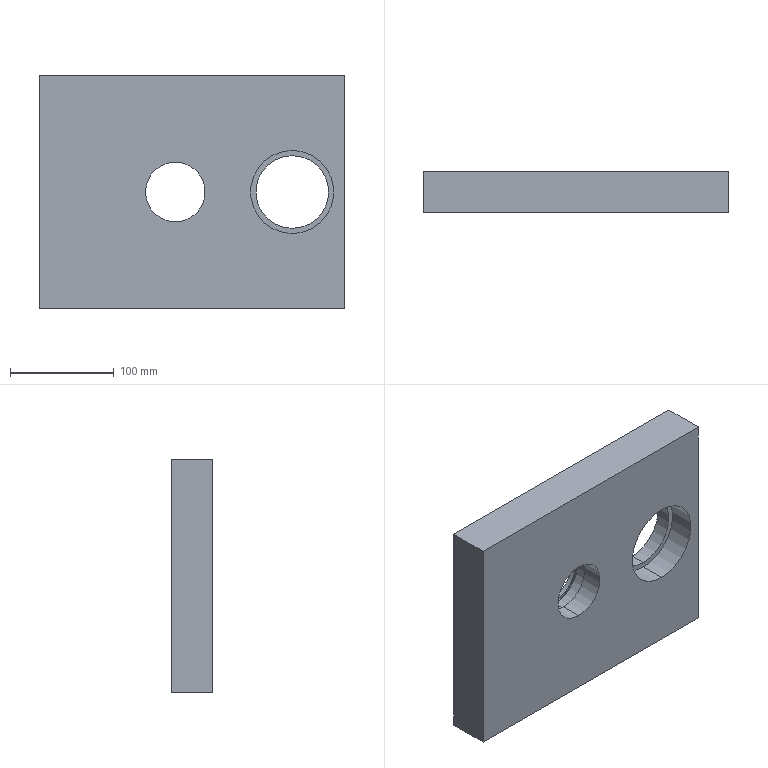Part | SolidWorks | features Cut 3, ICE 2, Extrusion 1 | 1 solid | 22 faces | box 293 x 40 x 225 mm | volume 2341161 mm3 | cylinder 12 | plane 10 | commonest cylinder face diameters 62 x4 57.4 x2 65 x2 70 x2 80 x2
STEP:
#1=CARTESIAN_POINT('',(-16.,32.8,-32.5));
#2=VERTEX_POINT('',#1);
#3=CARTESIAN_POINT('',(-16.,32.8,32.5));
#4=VERTEX_POINT('',#3);
#5=CARTESIAN_POINT('',(-16.,32.8,0.));
#6=DIRECTION('',(0.,1.,0.));
#7=DIRECTION('',(0.,0.,1.));
#8=AXIS2_PLACEMENT_3D('',#5,#6,#7);
#9=CIRCLE('',#8,32.5);
#10=EDGE_CURVE('',#2,#4,#9,.T.);
#11=ORIENTED_EDGE('',*,*,#10,.F.);
#12=CARTESIAN_POINT('',(-16.,35.,-32.5));
#13=VERTEX_POINT('',#12);
#14=CARTESIAN_POINT('',(-16.,32.8,-32.5));
#15=DIRECTION('',(0.,1.,0.));
#16=VECTOR('',#15,1000.);
#17=LINE('',#14,#16);
#18=EDGE_CURVE('',#2,#13,#17,.T.);
#19=ORIENTED_EDGE('',*,*,#18,.T.);
#20=CARTESIAN_POINT('',(-16.,35.,32.5));
#21=VERTEX_POINT('',#20);
#22=CARTESIAN_POINT('',(-16.,35.,0.));
#23=DIRECTION('',(0.,1.,0.));
#24=DIRECTION('',(0.,0.,1.));
#25=AXIS2_PLACEMENT_3D('',#22,#23,#24);
#26=CIRCLE('',#25,32.5);
#27=EDGE_CURVE('',#13,#21,#26,.T.);
#28=ORIENTED_EDGE('',*,*,#27,.T.);
#29=CARTESIAN_POINT('',(-16.,32.8,32.5));
#30=DIRECTION('',(0.,1.,0.));
#31=VECTOR('',#30,1000.);
#32=LINE('',#29,#31);
#33=EDGE_CURVE('',#4,#21,#32,.T.);
#34=ORIENTED_EDGE('',*,*,#33,.F.);
#35=EDGE_LOOP('',(#11,#19,#28,#34));
#36=FACE_OUTER_BOUND('',#35,.T.);
#37=CARTESIAN_POINT('',(-16.,32.8,0.));
#38=DIRECTION('',(0.,1.,0.));
#39=DIRECTION('',(0.,0.,1.));
#40=AXIS2_PLACEMENT_3D('',#37,#38,#39);
#41=CYLINDRICAL_SURFACE('',#40,32.5);
#42=ADVANCED_FACE('',(#36),#41,.F.);
#43=CARTESIAN_POINT('',(-16.,35.,31.));
#44=VERTEX_POINT('',#43);
#45=CARTESIAN_POINT('',(-16.,35.,-31.));
#46=VERTEX_POINT('',#45);
#47=CARTESIAN_POINT('',(-16.,35.,0.));
#48=DIRECTION('',(0.,-1.,0.));
#49=DIRECTION('',(0.,0.,1.));
#50=AXIS2_PLACEMENT_3D('',#47,#48,#49);
#51=CIRCLE('',#50,31.);
#52=EDGE_CURVE('',#44,#46,#51,.T.);
#53=ORIENTED_EDGE('',*,*,#52,.T.);
#54=CARTESIAN_POINT('',(-16.,40.,-31.));
#55=VERTEX_POINT('',#54);
#56=CARTESIAN_POINT('',(-16.,20.8,-31.));
#57=DIRECTION('',(0.,1.,0.));
#58=VECTOR('',#57,1000.);
#59=LINE('',#56,#58);
#60=EDGE_CURVE('',#46,#55,#59,.T.);
#61=ORIENTED_EDGE('',*,*,#60,.T.);
#62=CARTESIAN_POINT('',(-16.,40.,31.));
#63=VERTEX_POINT('',#62);
#64=CARTESIAN_POINT('',(-16.,40.,0.));
#65=DIRECTION('',(0.,1.,0.));
#66=DIRECTION('',(0.,0.,1.));
#67=AXIS2_PLACEMENT_3D('',#64,#65,#66);
#68=CIRCLE('',#67,31.);
#69=EDGE_CURVE('',#55,#63,#68,.T.);
#70=ORIENTED_EDGE('',*,*,#69,.T.);
#71=CARTESIAN_POINT('',(-16.,20.8,31.));
#72=DIRECTION('',(0.,1.,0.));
#73=VECTOR('',#72,1000.);
#74=LINE('',#71,#73);
#75=EDGE_CURVE('',#44,#63,#74,.T.);
#76=ORIENTED_EDGE('',*,*,#75,.F.);
#77=EDGE_LOOP('',(#53,#61,#70,#76));
#78=FACE_OUTER_BOUND('',#77,.T.);
#79=CARTESIAN_POINT('',(-16.,20.8,0.));
#80=DIRECTION('',(0.,1.,0.));
#81=DIRECTION('',(0.,0.,1.));
#82=AXIS2_PLACEMENT_3D('',#79,#80,#81);
#83=CYLINDRICAL_SURFACE('',#82,31.);
#84=ADVANCED_FACE('',(#78),#83,.F.);
#85=CARTESIAN_POINT('',(96.5,40.,35.));
#86=VERTEX_POINT('',#85);
#87=CARTESIAN_POINT('',(96.5,40.,-35.));
#88=VERTEX_POINT('',#87);
#89=CARTESIAN_POINT('',(96.5,40.,0.));
#90=DIRECTION('',(0.,-1.,0.));
#91=DIRECTION('',(0.,0.,-1.));
#92=AXIS2_PLACEMENT_3D('',#89,#90,#91);
#93=CIRCLE('',#92,35.);
#94=EDGE_CURVE('',#86,#88,#93,.T.);
#95=ORIENTED_EDGE('',*,*,#94,.F.);
#96=CARTESIAN_POINT('',(96.5,25.,35.));
#97=VERTEX_POINT('',#96);
#98=CARTESIAN_POINT('',(96.5,40.,35.));
#99=DIRECTION('',(0.,-1.,0.));
#100=VECTOR('',#99,1000.);
#101=LINE('',#98,#100);
#102=EDGE_CURVE('',#86,#97,#101,.T.);
#103=ORIENTED_EDGE('',*,*,#102,.T.);
#104=CARTESIAN_POINT('',(96.5,25.,-35.));
#105=VERTEX_POINT('',#104);
#106=CARTESIAN_POINT('',(96.5,25.,0.));
#107=DIRECTION('',(0.,-1.,0.));
#108=DIRECTION('',(0.,0.,-1.));
#109=AXIS2_PLACEMENT_3D('',#106,#107,#108);
#110=CIRCLE('',#109,35.);
#111=EDGE_CURVE('',#97,#105,#110,.T.);
#112=ORIENTED_EDGE('',*,*,#111,.T.);
#113=CARTESIAN_POINT('',(96.5,40.,-35.));
#114=DIRECTION('',(0.,-1.,0.));
#115=VECTOR('',#114,1000.);
#116=LINE('',#113,#115);
#117=EDGE_CURVE('',#88,#105,#116,.T.);
#118=ORIENTED_EDGE('',*,*,#117,.F.);
#119=EDGE_LOOP('',(#95,#103,#112,#118));
#120=FACE_OUTER_BOUND('',#119,.T.);
#121=CARTESIAN_POINT('',(96.5,40.,0.));
#122=DIRECTION('',(0.,-1.,0.));
#123=DIRECTION('',(0.,0.,-1.));
#124=AXIS2_PLACEMENT_3D('',#121,#122,#123);
#125=CYLINDRICAL_SURFACE('',#124,35.);
#126=ADVANCED_FACE('',(#120),#125,.F.);
#127=CARTESIAN_POINT('',(96.5,25.,40.));
#128=VERTEX_POINT('',#127);
#129=CARTESIAN_POINT('',(96.5,25.,-40.));
#130=VERTEX_POINT('',#129);
#131=CARTESIAN_POINT('',(96.5,25.,0.));
#132=DIRECTION('',(0.,-1.,0.));
#133=DIRECTION('',(0.,0.,-1.));
#134=AXIS2_PLACEMENT_3D('',#131,#132,#133);
#135=CIRCLE('',#134,40.);
#136=EDGE_CURVE('',#128,#130,#135,.T.);
#137=ORIENTED_EDGE('',*,*,#136,.F.);
#138=CARTESIAN_POINT('',(96.5,0.,40.));
#139=VERTEX_POINT('',#138);
#140=CARTESIAN_POINT('',(96.5,25.,40.));
#141=DIRECTION('',(0.,-1.,0.));
#142=VECTOR('',#141,1000.);
#143=LINE('',#140,#142);
#144=EDGE_CURVE('',#128,#139,#143,.T.);
#145=ORIENTED_EDGE('',*,*,#144,.T.);
#146=CARTESIAN_POINT('',(96.5,0.,-40.));
#147=VERTEX_POINT('',#146);
#148=CARTESIAN_POINT('',(96.5,0.,0.));
#149=DIRECTION('',(0.,-1.,0.));
#150=DIRECTION('',(0.,0.,-1.));
#151=AXIS2_PLACEMENT_3D('',#148,#149,#150);
#152=CIRCLE('',#151,40.);
#153=EDGE_CURVE('',#139,#147,#152,.T.);
#154=ORIENTED_EDGE('',*,*,#153,.T.);
#155=CARTESIAN_POINT('',(96.5,25.,-40.));
#156=DIRECTION('',(0.,-1.,0.));
#157=VECTOR('',#156,1000.);
#158=LINE('',#155,#157);
#159=EDGE_CURVE('',#130,#147,#158,.T.);
#160=ORIENTED_EDGE('',*,*,#159,.F.);
#161=EDGE_LOOP('',(#137,#145,#154,#160));
#162=FACE_OUTER_BOUND('',#161,.T.);
#163=CARTESIAN_POINT('',(96.5,25.,0.));
#164=DIRECTION('',(0.,-1.,0.));
#165=DIRECTION('',(0.,0.,-1.));
#166=AXIS2_PLACEMENT_3D('',#163,#164,#165);
#167=CYLINDRICAL_SURFACE('',#166,40.);
#168=ADVANCED_FACE('',(#162),#167,.F.);
#169=CARTESIAN_POINT('',(-16.,20.8,28.7));
#170=VERTEX_POINT('',#169);
#171=CARTESIAN_POINT('',(-16.,20.8,-28.7));
#172=VERTEX_POINT('',#171);
#173=CARTESIAN_POINT('',(-16.,20.8,0.));
#174=DIRECTION('',(0.,-1.,0.));
#175=DIRECTION('',(0.,0.,1.));
#176=AXIS2_PLACEMENT_3D('',#173,#174,#175);
#177=CIRCLE('',#176,28.7);
#178=EDGE_CURVE('',#170,#172,#177,.T.);
#179=ORIENTED_EDGE('',*,*,#178,.F.);
#180=CARTESIAN_POINT('',(-16.,0.,28.7));
#181=VERTEX_POINT('',#180);
#182=CARTESIAN_POINT('',(-16.,40.,28.7));
#183=DIRECTION('',(0.,-1.,0.));
#184=VECTOR('',#183,1000.);
#185=LINE('',#182,#184);
#186=EDGE_CURVE('',#170,#181,#185,.T.);
#187=ORIENTED_EDGE('',*,*,#186,.T.);
#188=CARTESIAN_POINT('',(-16.,0.,-28.7));
#189=VERTEX_POINT('',#188);
#190=CARTESIAN_POINT('',(-16.,0.,0.));
#191=DIRECTION('',(0.,-1.,0.));
#192=DIRECTION('',(0.,0.,-1.));
#193=AXIS2_PLACEMENT_3D('',#190,#191,#192);
#194=CIRCLE('',#193,28.7);
#195=EDGE_CURVE('',#181,#189,#194,.T.);
#196=ORIENTED_EDGE('',*,*,#195,.T.);
#197=CARTESIAN_POINT('',(-16.,40.,-28.7));
#198=DIRECTION('',(0.,-1.,0.));
#199=VECTOR('',#198,1000.);
#200=LINE('',#197,#199);
#201=EDGE_CURVE('',#172,#189,#200,.T.);
#202=ORIENTED_EDGE('',*,*,#201,.F.);
#203=EDGE_LOOP('',(#179,#187,#196,#202));
#204=FACE_OUTER_BOUND('',#203,.T.);
#205=CARTESIAN_POINT('',(-16.,40.,0.));
#206=DIRECTION('',(0.,-1.,0.));
#207=DIRECTION('',(0.,0.,-1.));
#208=AXIS2_PLACEMENT_3D('',#205,#206,#207);
#209=CYLINDRICAL_SURFACE('',#208,28.7);
#210=ADVANCED_FACE('',(#204),#209,.F.);
#211=CARTESIAN_POINT('',(-16.,20.8,-31.));
#212=VERTEX_POINT('',#211);
#213=CARTESIAN_POINT('',(-16.,20.8,31.));
#214=VERTEX_POINT('',#213);
#215=CARTESIAN_POINT('',(-16.,20.8,0.));
#216=DIRECTION('',(0.,1.,0.));
#217=DIRECTION('',(0.,0.,1.));
#218=AXIS2_PLACEMENT_3D('',#215,#216,#217);
#219=CIRCLE('',#218,31.);
#220=EDGE_CURVE('',#212,#214,#219,.T.);
#221=ORIENTED_EDGE('',*,*,#220,.F.);
#222=CARTESIAN_POINT('',(-16.,32.8,-31.));
#223=VERTEX_POINT('',#222);
#224=CARTESIAN_POINT('',(-16.,20.8,-31.));
#225=DIRECTION('',(0.,1.,0.));
#226=VECTOR('',#225,1000.);
#227=LINE('',#224,#226);
#228=EDGE_CURVE('',#212,#223,#227,.T.);
#229=ORIENTED_EDGE('',*,*,#228,.T.);
#230=CARTESIAN_POINT('',(-16.,32.8,31.));
#231=VERTEX_POINT('',#230);
#232=CARTESIAN_POINT('',(-16.,32.8,0.));
#233=DIRECTION('',(0.,-1.,0.));
#234=DIRECTION('',(0.,0.,1.));
#235=AXIS2_PLACEMENT_3D('',#232,#233,#234);
#236=CIRCLE('',#235,31.);
#237=EDGE_CURVE('',#231,#223,#236,.T.);
#238=ORIENTED_EDGE('',*,*,#237,.F.);
#239=CARTESIAN_POINT('',(-16.,20.8,31.));
#240=DIRECTION('',(0.,1.,0.));
#241=VECTOR('',#240,1000.);
#242=LINE('',#239,#241);
#243=EDGE_CURVE('',#214,#231,#242,.T.);
#244=ORIENTED_EDGE('',*,*,#243,.F.);
#245=EDGE_LOOP('',(#221,#229,#238,#244));
#246=FACE_OUTER_BOUND('',#245,.T.);
#247=CARTESIAN_POINT('',(-16.,20.8,0.));
#248=DIRECTION('',(0.,1.,0.));
#249=DIRECTION('',(0.,0.,1.));
#250=AXIS2_PLACEMENT_3D('',#247,#248,#249);
#251=CYLINDRICAL_SURFACE('',#250,31.);
#252=ADVANCED_FACE('',(#246),#251,.F.);
#253=ORIENTED_EDGE('',*,*,#228,.F.);
#254=CARTESIAN_POINT('',(-16.,20.8,0.));
#255=DIRECTION('',(0.,1.,0.));
#256=DIRECTION('',(0.,0.,1.));
#257=AXIS2_PLACEMENT_3D('',#254,#255,#256);
#258=CIRCLE('',#257,31.);
#259=EDGE_CURVE('',#214,#212,#258,.T.);
#260=ORIENTED_EDGE('',*,*,#259,.F.);
#261=ORIENTED_EDGE('',*,*,#243,.T.);
#262=CARTESIAN_POINT('',(-16.,32.8,0.));
#263=DIRECTION('',(0.,-1.,0.));
#264=DIRECTION('',(0.,0.,1.));
#265=AXIS2_PLACEMENT_3D('',#262,#263,#264);
#266=CIRCLE('',#265,31.);
#267=EDGE_CURVE('',#223,#231,#266,.T.);
#268=ORIENTED_EDGE('',*,*,#267,.F.);
#269=EDGE_LOOP('',(#253,#260,#261,#268));
#270=FACE_OUTER_BOUND('',#269,.T.);
#271=CARTESIAN_POINT('',(-16.,20.8,0.));
#272=DIRECTION('',(0.,1.,0.));
#273=DIRECTION('',(0.,0.,1.));
#274=AXIS2_PLACEMENT_3D('',#271,#272,#273);
#275=CYLINDRICAL_SURFACE('',#274,31.);
#276=ADVANCED_FACE('',(#270),#275,.F.);
#277=ORIENTED_EDGE('',*,*,#186,.F.);
#278=CARTESIAN_POINT('',(-16.,20.8,0.));
#279=DIRECTION('',(0.,-1.,0.));
#280=DIRECTION('',(0.,0.,1.));
#281=AXIS2_PLACEMENT_3D('',#278,#279,#280);
#282=CIRCLE('',#281,28.7);
#283=EDGE_CURVE('',#172,#170,#282,.T.);
#284=ORIENTED_EDGE('',*,*,#283,.F.);
#285=ORIENTED_EDGE('',*,*,#201,.T.);
#286=CARTESIAN_POINT('',(-16.,0.,0.));
#287=DIRECTION('',(0.,-1.,0.));
#288=DIRECTION('',(0.,0.,-1.));
#289=AXIS2_PLACEMENT_3D('',#286,#287,#288);
#290=CIRCLE('',#289,28.7);
#291=EDGE_CURVE('',#189,#181,#290,.T.);
#292=ORIENTED_EDGE('',*,*,#291,.T.);
#293=EDGE_LOOP('',(#277,#284,#285,#292));
#294=FACE_OUTER_BOUND('',#293,.T.);
#295=CARTESIAN_POINT('',(-16.,40.,0.));
#296=DIRECTION('',(0.,-1.,0.));
#297=DIRECTION('',(0.,0.,-1.));
#298=AXIS2_PLACEMENT_3D('',#295,#296,#297);
#299=CYLINDRICAL_SURFACE('',#298,28.7);
#300=ADVANCED_FACE('',(#294),#299,.F.);
#301=CARTESIAN_POINT('',(146.5,0.,112.5));
#302=VERTEX_POINT('',#301);
#303=CARTESIAN_POINT('',(146.5,0.,-112.5));
#304=VERTEX_POINT('',#303);
#305=CARTESIAN_POINT('',(146.5,0.,112.5));
#306=DIRECTION('',(0.,0.,-1.));
#307=VECTOR('',#306,1000.);
#308=LINE('',#305,#307);
#309=EDGE_CURVE('',#302,#304,#308,.T.);
#310=ORIENTED_EDGE('',*,*,#309,.T.);
#311=CARTESIAN_POINT('',(146.5,40.,-112.5));
#312=VERTEX_POINT('',#311);
#313=CARTESIAN_POINT('',(146.5,40.,-112.5));
#314=DIRECTION('',(0.,-1.,0.));
#315=VECTOR('',#314,1000.);
#316=LINE('',#313,#315);
#317=EDGE_CURVE('',#312,#304,#316,.T.);
#318=ORIENTED_EDGE('',*,*,#317,.F.);
#319=CARTESIAN_POINT('',(146.5,40.,112.5));
#320=VERTEX_POINT('',#319);
#321=CARTESIAN_POINT('',(146.5,40.,112.5));
#322=DIRECTION('',(0.,0.,-1.));
#323=VECTOR('',#322,1000.);
#324=LINE('',#321,#323);
#325=EDGE_CURVE('',#320,#312,#324,.T.);
#326=ORIENTED_EDGE('',*,*,#325,.F.);
#327=CARTESIAN_POINT('',(146.5,40.,112.5));
#328=DIRECTION('',(0.,-1.,0.));
#329=VECTOR('',#328,1000.);
#330=LINE('',#327,#329);
#331=EDGE_CURVE('',#320,#302,#330,.T.);
#332=ORIENTED_EDGE('',*,*,#331,.T.);
#333=EDGE_LOOP('',(#310,#318,#326,#332));
#334=FACE_OUTER_BOUND('',#333,.T.);
#335=CARTESIAN_POINT('',(146.5,40.,112.5));
#336=DIRECTION('',(-1.,0.,0.));
#337=DIRECTION('',(0.,0.,1.));
#338=AXIS2_PLACEMENT_3D('',#335,#336,#337);
#339=PLANE('',#338);
#340=ADVANCED_FACE('',(#334),#339,.F.);
#341=CARTESIAN_POINT('',(-146.5,0.,-112.5));
#342=VERTEX_POINT('',#341);
#343=CARTESIAN_POINT('',(-146.5,0.,-112.5));
#344=DIRECTION('',(-1.,0.,0.));
#345=VECTOR('',#344,1000.);
#346=LINE('',#343,#345);
#347=EDGE_CURVE('',#304,#342,#346,.T.);
#348=ORIENTED_EDGE('',*,*,#347,.T.);
#349=CARTESIAN_POINT('',(-146.5,40.,-112.5));
#350=VERTEX_POINT('',#349);
#351=CARTESIAN_POINT('',(-146.5,40.,-112.5));
#352=DIRECTION('',(0.,-1.,0.));
#353=VECTOR('',#352,1000.);
#354=LINE('',#351,#353);
#355=EDGE_CURVE('',#350,#342,#354,.T.);
#356=ORIENTED_EDGE('',*,*,#355,.F.);
#357=CARTESIAN_POINT('',(-146.5,40.,-112.5));
#358=DIRECTION('',(-1.,0.,0.));
#359=VECTOR('',#358,1000.);
#360=LINE('',#357,#359);
#361=EDGE_CURVE('',#312,#350,#360,.T.);
#362=ORIENTED_EDGE('',*,*,#361,.F.);
#363=ORIENTED_EDGE('',*,*,#317,.T.);
#364=EDGE_LOOP('',(#348,#356,#362,#363));
#365=FACE_OUTER_BOUND('',#364,.T.);
#366=CARTESIAN_POINT('',(-146.5,40.,-112.5));
#367=DIRECTION('',(0.,0.,1.));
#368=DIRECTION('',(1.,0.,0.));
#369=AXIS2_PLACEMENT_3D('',#366,#367,#368);
#370=PLANE('',#369);
#371=ADVANCED_FACE('',(#365),#370,.F.);
#372=CARTESIAN_POINT('',(-146.5,0.,112.5));
#373=VERTEX_POINT('',#372);
#374=CARTESIAN_POINT('',(-146.5,0.,112.5));
#375=DIRECTION('',(0.,0.,1.));
#376=VECTOR('',#375,1000.);
#377=LINE('',#374,#376);
#378=EDGE_CURVE('',#342,#373,#377,.T.);
#379=ORIENTED_EDGE('',*,*,#378,.T.);
#380=CARTESIAN_POINT('',(-146.5,40.,112.5));
#381=VERTEX_POINT('',#380);
#382=CARTESIAN_POINT('',(-146.5,40.,112.5));
#383=DIRECTION('',(0.,-1.,0.));
#384=VECTOR('',#383,1000.);
#385=LINE('',#382,#384);
#386=EDGE_CURVE('',#381,#373,#385,.T.);
#387=ORIENTED_EDGE('',*,*,#386,.F.);
#388=CARTESIAN_POINT('',(-146.5,40.,112.5));
#389=DIRECTION('',(0.,0.,1.));
#390=VECTOR('',#389,1000.);
#391=LINE('',#388,#390);
#392=EDGE_CURVE('',#350,#381,#391,.T.);
#393=ORIENTED_EDGE('',*,*,#392,.F.);
#394=ORIENTED_EDGE('',*,*,#355,.T.);
#395=EDGE_LOOP('',(#379,#387,#393,#394));
#396=FACE_OUTER_BOUND('',#395,.T.);
#397=CARTESIAN_POINT('',(-146.5,40.,112.5));
#398=DIRECTION('',(1.,0.,0.));
#399=DIRECTION('',(0.,0.,-1.));
#400=AXIS2_PLACEMENT_3D('',#397,#398,#399);
#401=PLANE('',#400);
#402=ADVANCED_FACE('',(#396),#401,.F.);
#403=CARTESIAN_POINT('',(-146.5,0.,112.5));
#404=DIRECTION('',(1.,0.,0.));
#405=VECTOR('',#404,1000.);
#406=LINE('',#403,#405);
#407=EDGE_CURVE('',#373,#302,#406,.T.);
#408=ORIENTED_EDGE('',*,*,#407,.T.);
#409=ORIENTED_EDGE('',*,*,#331,.F.);
#410=CARTESIAN_POINT('',(-146.5,40.,112.5));
#411=DIRECTION('',(1.,0.,0.));
#412=VECTOR('',#411,1000.);
#413=LINE('',#410,#412);
#414=EDGE_CURVE('',#381,#320,#413,.T.);
#415=ORIENTED_EDGE('',*,*,#414,.F.);
#416=ORIENTED_EDGE('',*,*,#386,.T.);
#417=EDGE_LOOP('',(#408,#409,#415,#416));
#418=FACE_OUTER_BOUND('',#417,.T.);
#419=CARTESIAN_POINT('',(-146.5,40.,112.5));
#420=DIRECTION('',(0.,0.,-1.));
#421=DIRECTION('',(-1.,0.,0.));
#422=AXIS2_PLACEMENT_3D('',#419,#420,#421);
#423=PLANE('',#422);
#424=ADVANCED_FACE('',(#418),#423,.F.);
#425=CARTESIAN_POINT('',(-16.,40.,0.));
#426=DIRECTION('',(0.,1.,0.));
#427=DIRECTION('',(0.,0.,1.));
#428=AXIS2_PLACEMENT_3D('',#425,#426,#427);
#429=CIRCLE('',#428,31.);
#430=EDGE_CURVE('',#63,#55,#429,.T.);
#431=ORIENTED_EDGE('',*,*,#430,.F.);
#432=ORIENTED_EDGE('',*,*,#69,.F.);
#433=EDGE_LOOP('',(#431,#432));
#434=FACE_BOUND('',#433,.T.);
#435=CARTESIAN_POINT('',(96.5,40.,0.));
#436=DIRECTION('',(0.,-1.,0.));
#437=DIRECTION('',(0.,0.,-1.));
#438=AXIS2_PLACEMENT_3D('',#435,#436,#437);
#439=CIRCLE('',#438,35.);
#440=EDGE_CURVE('',#88,#86,#439,.T.);
#441=ORIENTED_EDGE('',*,*,#440,.T.);
#442=ORIENTED_EDGE('',*,*,#94,.T.);
#443=EDGE_LOOP('',(#441,#442));
#444=FACE_BOUND('',#443,.T.);
#445=ORIENTED_EDGE('',*,*,#325,.T.);
#446=ORIENTED_EDGE('',*,*,#361,.T.);
#447=ORIENTED_EDGE('',*,*,#392,.T.);
#448=ORIENTED_EDGE('',*,*,#414,.T.);
#449=EDGE_LOOP('',(#445,#446,#447,#448));
#450=FACE_OUTER_BOUND('',#449,.T.);
#451=CARTESIAN_POINT('',(0.,40.,0.));
#452=DIRECTION('',(0.,-1.,0.));
#453=DIRECTION('',(0.,0.,-1.));
#454=AXIS2_PLACEMENT_3D('',#451,#452,#453);
#455=PLANE('',#454);
#456=ADVANCED_FACE('',(#434,#444,#450),#455,.F.);
#457=ORIENTED_EDGE('',*,*,#291,.F.);
#458=ORIENTED_EDGE('',*,*,#195,.F.);
#459=EDGE_LOOP('',(#457,#458));
#460=FACE_BOUND('',#459,.T.);
#461=CARTESIAN_POINT('',(96.5,0.,0.));
#462=DIRECTION('',(0.,-1.,0.));
#463=DIRECTION('',(0.,0.,-1.));
#464=AXIS2_PLACEMENT_3D('',#461,#462,#463);
#465=CIRCLE('',#464,40.);
#466=EDGE_CURVE('',#147,#139,#465,.T.);
#467=ORIENTED_EDGE('',*,*,#466,.F.);
#468=ORIENTED_EDGE('',*,*,#153,.F.);
#469=EDGE_LOOP('',(#467,#468));
#470=FACE_BOUND('',#469,.T.);
#471=ORIENTED_EDGE('',*,*,#309,.F.);
#472=ORIENTED_EDGE('',*,*,#407,.F.);
#473=ORIENTED_EDGE('',*,*,#378,.F.);
#474=ORIENTED_EDGE('',*,*,#347,.F.);
#475=EDGE_LOOP('',(#471,#472,#473,#474));
#476=FACE_OUTER_BOUND('',#475,.T.);
#477=CARTESIAN_POINT('',(0.,0.,0.));
#478=DIRECTION('',(0.,-1.,0.));
#479=DIRECTION('',(0.,0.,-1.));
#480=AXIS2_PLACEMENT_3D('',#477,#478,#479);
#481=PLANE('',#480);
#482=ADVANCED_FACE('',(#460,#470,#476),#481,.T.);
#483=ORIENTED_EDGE('',*,*,#144,.F.);
#484=CARTESIAN_POINT('',(96.5,25.,0.));
#485=DIRECTION('',(0.,-1.,0.));
#486=DIRECTION('',(0.,0.,-1.));
#487=AXIS2_PLACEMENT_3D('',#484,#485,#486);
#488=CIRCLE('',#487,40.);
#489=EDGE_CURVE('',#130,#128,#488,.T.);
#490=ORIENTED_EDGE('',*,*,#489,.F.);
#491=ORIENTED_EDGE('',*,*,#159,.T.);
#492=ORIENTED_EDGE('',*,*,#466,.T.);
#493=EDGE_LOOP('',(#483,#490,#491,#492));
#494=FACE_OUTER_BOUND('',#493,.T.);
#495=CARTESIAN_POINT('',(96.5,25.,0.));
#496=DIRECTION('',(0.,-1.,0.));
#497=DIRECTION('',(0.,0.,-1.));
#498=AXIS2_PLACEMENT_3D('',#495,#496,#497);
#499=CYLINDRICAL_SURFACE('',#498,40.);
#500=ADVANCED_FACE('',(#494),#499,.F.);
#501=CARTESIAN_POINT('',(96.5,25.,0.));
#502=DIRECTION('',(0.,-1.,0.));
#503=DIRECTION('',(0.,0.,-1.));
#504=AXIS2_PLACEMENT_3D('',#501,#502,#503);
#505=CIRCLE('',#504,35.);
#506=EDGE_CURVE('',#105,#97,#505,.T.);
#507=ORIENTED_EDGE('',*,*,#506,.F.);
#508=ORIENTED_EDGE('',*,*,#111,.F.);
#509=EDGE_LOOP('',(#507,#508));
#510=FACE_BOUND('',#509,.T.);
#511=ORIENTED_EDGE('',*,*,#489,.T.);
#512=ORIENTED_EDGE('',*,*,#136,.T.);
#513=EDGE_LOOP('',(#511,#512));
#514=FACE_OUTER_BOUND('',#513,.T.);
#515=CARTESIAN_POINT('',(96.5,25.,0.));
#516=DIRECTION('',(0.,-1.,0.));
#517=DIRECTION('',(0.,0.,-1.));
#518=AXIS2_PLACEMENT_3D('',#515,#516,#517);
#519=PLANE('',#518);
#520=ADVANCED_FACE('',(#510,#514),#519,.T.);
#521=ORIENTED_EDGE('',*,*,#102,.F.);
#522=ORIENTED_EDGE('',*,*,#440,.F.);
#523=ORIENTED_EDGE('',*,*,#117,.T.);
#524=ORIENTED_EDGE('',*,*,#506,.T.);
#525=EDGE_LOOP('',(#521,#522,#523,#524));
#526=FACE_OUTER_BOUND('',#525,.T.);
#527=CARTESIAN_POINT('',(96.5,40.,0.));
#528=DIRECTION('',(0.,-1.,0.));
#529=DIRECTION('',(0.,0.,-1.));
#530=AXIS2_PLACEMENT_3D('',#527,#528,#529);
#531=CYLINDRICAL_SURFACE('',#530,35.);
#532=ADVANCED_FACE('',(#526),#531,.F.);
#533=ORIENTED_EDGE('',*,*,#259,.T.);
#534=ORIENTED_EDGE('',*,*,#220,.T.);
#535=EDGE_LOOP('',(#533,#534));
#536=FACE_OUTER_BOUND('',#535,.T.);
#537=ORIENTED_EDGE('',*,*,#283,.T.);
#538=ORIENTED_EDGE('',*,*,#178,.T.);
#539=EDGE_LOOP('',(#537,#538));
#540=FACE_BOUND('',#539,.T.);
#541=CARTESIAN_POINT('',(-16.,20.8,0.));
#542=DIRECTION('',(0.,1.,0.));
#543=DIRECTION('',(0.,0.,1.));
#544=AXIS2_PLACEMENT_3D('',#541,#542,#543);
#545=PLANE('',#544);
#546=ADVANCED_FACE('',(#536,#540),#545,.T.);
#547=ORIENTED_EDGE('',*,*,#60,.F.);
#548=CARTESIAN_POINT('',(-16.,35.,0.));
#549=DIRECTION('',(0.,-1.,0.));
#550=DIRECTION('',(0.,0.,1.));
#551=AXIS2_PLACEMENT_3D('',#548,#549,#550);
#552=CIRCLE('',#551,31.);
#553=EDGE_CURVE('',#46,#44,#552,.T.);
#554=ORIENTED_EDGE('',*,*,#553,.T.);
#555=ORIENTED_EDGE('',*,*,#75,.T.);
#556=ORIENTED_EDGE('',*,*,#430,.T.);
#557=EDGE_LOOP('',(#547,#554,#555,#556));
#558=FACE_OUTER_BOUND('',#557,.T.);
#559=CARTESIAN_POINT('',(-16.,20.8,0.));
#560=DIRECTION('',(0.,1.,0.));
#561=DIRECTION('',(0.,0.,1.));
#562=AXIS2_PLACEMENT_3D('',#559,#560,#561);
#563=CYLINDRICAL_SURFACE('',#562,31.);
#564=ADVANCED_FACE('',(#558),#563,.F.);
#565=CARTESIAN_POINT('',(-16.,32.8,0.));
#566=DIRECTION('',(0.,1.,0.));
#567=DIRECTION('',(0.,0.,1.));
#568=AXIS2_PLACEMENT_3D('',#565,#566,#567);
#569=CIRCLE('',#568,32.5);
#570=EDGE_CURVE('',#4,#2,#569,.T.);
#571=ORIENTED_EDGE('',*,*,#570,.T.);
#572=ORIENTED_EDGE('',*,*,#10,.T.);
#573=EDGE_LOOP('',(#571,#572));
#574=FACE_OUTER_BOUND('',#573,.T.);
#575=ORIENTED_EDGE('',*,*,#237,.T.);
#576=ORIENTED_EDGE('',*,*,#267,.T.);
#577=EDGE_LOOP('',(#575,#576));
#578=FACE_BOUND('',#577,.T.);
#579=CARTESIAN_POINT('',(-16.,32.8,0.));
#580=DIRECTION('',(0.,1.,0.));
#581=DIRECTION('',(0.,0.,1.));
#582=AXIS2_PLACEMENT_3D('',#579,#580,#581);
#583=PLANE('',#582);
#584=ADVANCED_FACE('',(#574,#578),#583,.T.);
#585=CARTESIAN_POINT('',(-16.,35.,0.));
#586=DIRECTION('',(0.,1.,0.));
#587=DIRECTION('',(0.,0.,1.));
#588=AXIS2_PLACEMENT_3D('',#585,#586,#587);
#589=CIRCLE('',#588,32.5);
#590=EDGE_CURVE('',#21,#13,#589,.T.);
#591=ORIENTED_EDGE('',*,*,#590,.F.);
#592=ORIENTED_EDGE('',*,*,#27,.F.);
#593=EDGE_LOOP('',(#591,#592));
#594=FACE_OUTER_BOUND('',#593,.T.);
#595=ORIENTED_EDGE('',*,*,#52,.F.);
#596=ORIENTED_EDGE('',*,*,#553,.F.);
#597=EDGE_LOOP('',(#595,#596));
#598=FACE_BOUND('',#597,.T.);
#599=CARTESIAN_POINT('',(-16.,35.,0.));
#600=DIRECTION('',(0.,1.,0.));
#601=DIRECTION('',(0.,0.,1.));
#602=AXIS2_PLACEMENT_3D('',#599,#600,#601);
#603=PLANE('',#602);
#604=ADVANCED_FACE('',(#594,#598),#603,.F.);
#605=ORIENTED_EDGE('',*,*,#18,.F.);
#606=ORIENTED_EDGE('',*,*,#570,.F.);
#607=ORIENTED_EDGE('',*,*,#33,.T.);
#608=ORIENTED_EDGE('',*,*,#590,.T.);
#609=EDGE_LOOP('',(#605,#606,#607,#608));
#610=FACE_OUTER_BOUND('',#609,.T.);
#611=CARTESIAN_POINT('',(-16.,32.8,0.));
#612=DIRECTION('',(0.,1.,0.));
#613=DIRECTION('',(0.,0.,1.));
#614=AXIS2_PLACEMENT_3D('',#611,#612,#613);
#615=CYLINDRICAL_SURFACE('',#614,32.5);
#616=ADVANCED_FACE('',(#610),#615,.F.);
#617=CLOSED_SHELL('',(#42,#84,#126,#168,#210,#252,#276,#300,#340,#371,#402,#424,#456,#482,#500,#520,#532,#546,#564,#584,#604,#616));
#618=MANIFOLD_SOLID_BREP('',#617);
#619=CARTESIAN_POINT('',(0.,0.,0.));
#620=DIRECTION('',(0.,0.,1.));
#621=DIRECTION('',(1.,0.,0.));
#622=AXIS2_PLACEMENT_3D('',#619,#620,#621);
#623=(LENGTH_UNIT()NAMED_UNIT(*)SI_UNIT(.MILLI.,.METRE.));
#624=UNCERTAINTY_MEASURE_WITH_UNIT(LENGTH_MEASURE(0.00001),#623,'','');
#625=(NAMED_UNIT(*)PLANE_ANGLE_UNIT()SI_UNIT($,.RADIAN.));
#626=(NAMED_UNIT(*)SI_UNIT($,.STERADIAN.)SOLID_ANGLE_UNIT());
#627=(GEOMETRIC_REPRESENTATION_CONTEXT(3)GLOBAL_UNCERTAINTY_ASSIGNED_CONTEXT((#624))GLOBAL_UNIT_ASSIGNED_CONTEXT((#623,#625,#626))REPRESENTATION_CONTEXT('',''));
#628=ADVANCED_BREP_SHAPE_REPRESENTATION('',(#618,#622),#627);